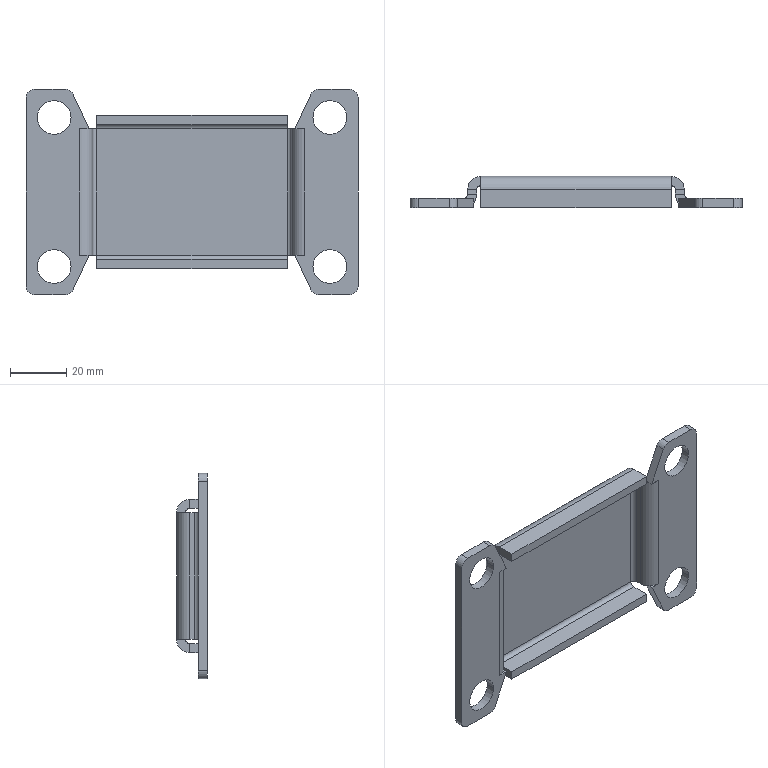Part | STEP file | VBA22A-03GN_VBA20A Bracket | 1 solid | 78 faces | box 118 x 11 x 73 mm | volume 25260 mm3 | plane 50 | cylinder 28 | commonest cylinder face diameters 6 x8 12 x8 3 x6 9.4 x6